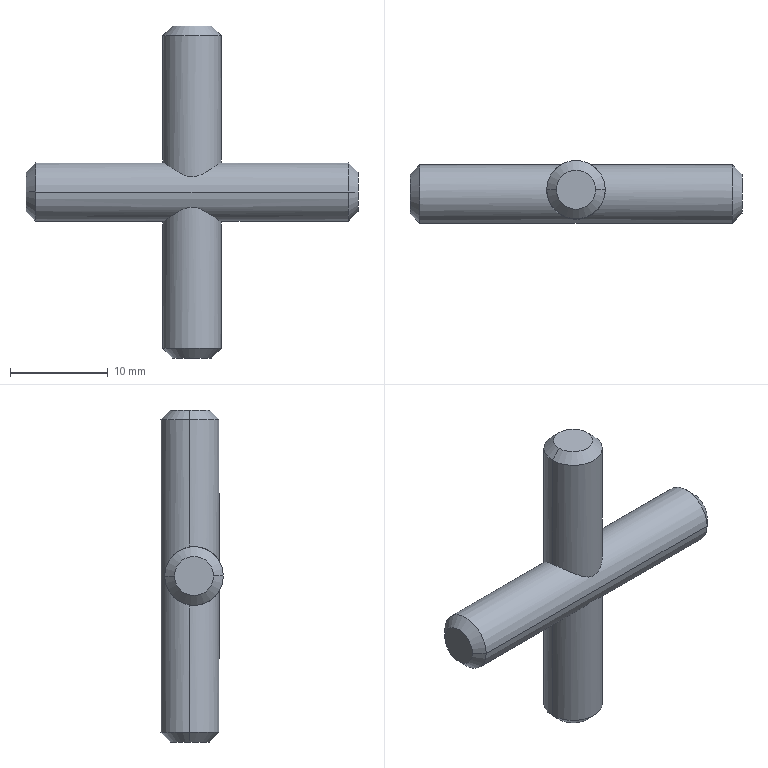Part | SolidWorks | features MBimport 1 | 1 solid | 17 faces | box 34 x 6.427 x 34 mm | volume 1749 mm3 | cone 8 | cylinder 5 | plane 4 | commonest cylinder face diameters 6 x5
STEP:
#1=CARTESIAN_POINT('',(14.,0.4269,-16.));
#2=VERTEX_POINT('',#1);
#3=CARTESIAN_POINT('',(15.,0.4269,-17.));
#4=VERTEX_POINT('',#3);
#5=CARTESIAN_POINT('',(14.5,0.4269,-16.5));
#6=DIRECTION('',(0.7071,-0.000000084,-0.7071));
#7=VECTOR('',#6,1000.);
#8=LINE('',#5,#7);
#9=EDGE_CURVE('',#2,#4,#8,.T.);
#10=ORIENTED_EDGE('',*,*,#9,.T.);
#11=CARTESIAN_POINT('',(19.,0.4269,-17.));
#12=VERTEX_POINT('',#11);
#13=CARTESIAN_POINT('',(17.,0.4269,-17.));
#14=DIRECTION('',(0.,0.,1.));
#15=DIRECTION('',(1.,0.,0.));
#16=AXIS2_PLACEMENT_3D('',#13,#14,#15);
#17=CIRCLE('',#16,2.);
#18=EDGE_CURVE('',#4,#12,#17,.T.);
#19=ORIENTED_EDGE('',*,*,#18,.T.);
#20=CARTESIAN_POINT('',(20.,0.4269,-16.));
#21=VERTEX_POINT('',#20);
#22=CARTESIAN_POINT('',(19.5,0.4269,-16.5));
#23=DIRECTION('',(-0.7071,0.,-0.7071));
#24=VECTOR('',#23,1000.);
#25=LINE('',#22,#24);
#26=EDGE_CURVE('',#21,#12,#25,.T.);
#27=ORIENTED_EDGE('',*,*,#26,.F.);
#28=CARTESIAN_POINT('',(17.,0.4269,-16.));
#29=DIRECTION('',(0.,0.,1.));
#30=DIRECTION('',(1.,0.,0.));
#31=AXIS2_PLACEMENT_3D('',#28,#29,#30);
#32=CIRCLE('',#31,3.);
#33=EDGE_CURVE('',#2,#21,#32,.T.);
#34=ORIENTED_EDGE('',*,*,#33,.F.);
#35=EDGE_LOOP('',(#10,#19,#27,#34));
#36=FACE_OUTER_BOUND('',#35,.T.);
#37=CARTESIAN_POINT('',(17.,0.4269,-18.));
#38=DIRECTION('',(0.,0.,1.));
#39=DIRECTION('',(-0.9607,0.2774,0.));
#40=AXIS2_PLACEMENT_3D('',#37,#38,#39);
#41=CONICAL_SURFACE('',#40,1.,0.7854);
#42=ADVANCED_FACE('',(#36),#41,.T.);
#43=ORIENTED_EDGE('',*,*,#26,.T.);
#44=CARTESIAN_POINT('',(17.,0.4269,-17.));
#45=DIRECTION('',(0.,0.,1.));
#46=DIRECTION('',(1.,0.,0.));
#47=AXIS2_PLACEMENT_3D('',#44,#45,#46);
#48=CIRCLE('',#47,2.);
#49=EDGE_CURVE('',#12,#4,#48,.T.);
#50=ORIENTED_EDGE('',*,*,#49,.T.);
#51=ORIENTED_EDGE('',*,*,#9,.F.);
#52=CARTESIAN_POINT('',(17.,0.4269,-16.));
#53=DIRECTION('',(0.,0.,1.));
#54=DIRECTION('',(1.,0.,0.));
#55=AXIS2_PLACEMENT_3D('',#52,#53,#54);
#56=CIRCLE('',#55,3.);
#57=EDGE_CURVE('',#21,#2,#56,.T.);
#58=ORIENTED_EDGE('',*,*,#57,.F.);
#59=EDGE_LOOP('',(#43,#50,#51,#58));
#60=FACE_OUTER_BOUND('',#59,.T.);
#61=CARTESIAN_POINT('',(17.,0.4269,-18.));
#62=DIRECTION('',(0.,0.,1.));
#63=DIRECTION('',(1.,0.,0.));
#64=AXIS2_PLACEMENT_3D('',#61,#62,#63);
#65=CONICAL_SURFACE('',#64,1.,0.7854);
#66=ADVANCED_FACE('',(#60),#65,.T.);
#67=CARTESIAN_POINT('',(14.,0.4269,-2.969));
#68=VERTEX_POINT('',#67);
#69=CARTESIAN_POINT('',(14.,0.4269,0.));
#70=DIRECTION('',(0.,0.,1.));
#71=VECTOR('',#70,1000.);
#72=LINE('',#69,#71);
#73=EDGE_CURVE('',#2,#68,#72,.T.);
#74=ORIENTED_EDGE('',*,*,#73,.T.);
#75=CARTESIAN_POINT('',(15.458,3.,0.));
#76=VERTEX_POINT('',#75);
#77=CARTESIAN_POINT('',(15.458,3.,0.));
#78=CARTESIAN_POINT('',(15.458,3.,-0.1084));
#79=CARTESIAN_POINT('',(15.449,2.995,-0.2169));
#80=CARTESIAN_POINT('',(15.433,2.985,-0.324));
#81=CARTESIAN_POINT('',(15.385,2.956,-0.541));
#82=CARTESIAN_POINT('',(15.313,2.908,-0.748));
#83=CARTESIAN_POINT('',(15.271,2.879,-0.8517));
#84=CARTESIAN_POINT('',(15.169,2.806,-1.078));
#85=CARTESIAN_POINT('',(15.055,2.713,-1.29));
#86=CARTESIAN_POINT('',(14.989,2.656,-1.404));
#87=CARTESIAN_POINT('',(14.832,2.508,-1.662));
#88=CARTESIAN_POINT('',(14.675,2.33,-1.901));
#89=CARTESIAN_POINT('',(14.587,2.218,-2.031));
#90=CARTESIAN_POINT('',(14.445,2.013,-2.237));
#91=CARTESIAN_POINT('',(14.319,1.779,-2.42));
#92=CARTESIAN_POINT('',(14.271,1.68,-2.49));
#93=CARTESIAN_POINT('',(14.182,1.472,-2.621));
#94=CARTESIAN_POINT('',(14.111,1.248,-2.733));
#95=CARTESIAN_POINT('',(14.08,1.131,-2.783));
#96=CARTESIAN_POINT('',(14.036,0.9238,-2.86));
#97=CARTESIAN_POINT('',(14.011,0.7074,-2.918));
#98=CARTESIAN_POINT('',(14.004,0.6147,-2.939));
#99=CARTESIAN_POINT('',(14.,0.5211,-2.956));
#100=CARTESIAN_POINT('',(14.,0.4269,-2.969));
#101=B_SPLINE_CURVE_WITH_KNOTS('',5,(#77,#78,#79,#80,#81,#82,#83,#84,#85,#86,#87,#88,#89,#90,#91,#92,#93,#94,#95,#96,#97,#98,#99,#100),.UNSPECIFIED.,.F.,.F.,(6,3,3,3,3,3,3,6),(0.,0.7667,1.581,2.593,3.956,4.875,5.794,6.467),.UNSPECIFIED.);
#102=EDGE_CURVE('',#76,#68,#101,.T.);
#103=ORIENTED_EDGE('',*,*,#102,.F.);
#104=CARTESIAN_POINT('',(14.,0.4269,2.969));
#105=VERTEX_POINT('',#104);
#106=CARTESIAN_POINT('',(15.458,3.,0.));
#107=CARTESIAN_POINT('',(15.458,3.,0.1084));
#108=CARTESIAN_POINT('',(15.449,2.995,0.2169));
#109=CARTESIAN_POINT('',(15.433,2.985,0.324));
#110=CARTESIAN_POINT('',(15.385,2.956,0.541));
#111=CARTESIAN_POINT('',(15.313,2.908,0.748));
#112=CARTESIAN_POINT('',(15.271,2.879,0.8517));
#113=CARTESIAN_POINT('',(15.169,2.806,1.078));
#114=CARTESIAN_POINT('',(15.055,2.713,1.29));
#115=CARTESIAN_POINT('',(14.989,2.656,1.404));
#116=CARTESIAN_POINT('',(14.832,2.508,1.662));
#117=CARTESIAN_POINT('',(14.675,2.33,1.901));
#118=CARTESIAN_POINT('',(14.587,2.218,2.031));
#119=CARTESIAN_POINT('',(14.445,2.013,2.237));
#120=CARTESIAN_POINT('',(14.319,1.779,2.42));
#121=CARTESIAN_POINT('',(14.271,1.68,2.49));
#122=CARTESIAN_POINT('',(14.182,1.472,2.621));
#123=CARTESIAN_POINT('',(14.111,1.248,2.733));
#124=CARTESIAN_POINT('',(14.08,1.131,2.783));
#125=CARTESIAN_POINT('',(14.036,0.9238,2.86));
#126=CARTESIAN_POINT('',(14.011,0.7074,2.918));
#127=CARTESIAN_POINT('',(14.004,0.6147,2.939));
#128=CARTESIAN_POINT('',(14.,0.5211,2.956));
#129=CARTESIAN_POINT('',(14.,0.4269,2.969));
#130=B_SPLINE_CURVE_WITH_KNOTS('',5,(#106,#107,#108,#109,#110,#111,#112,#113,#114,#115,#116,#117,#118,#119,#120,#121,#122,#123,#124,#125,#126,#127,#128,#129),.UNSPECIFIED.,.F.,.F.,(6,3,3,3,3,3,3,6),(0.,0.7667,1.581,2.593,3.956,4.875,5.794,6.467),.UNSPECIFIED.);
#131=EDGE_CURVE('',#76,#105,#130,.T.);
#132=ORIENTED_EDGE('',*,*,#131,.T.);
#133=CARTESIAN_POINT('',(14.,0.4269,16.));
#134=VERTEX_POINT('',#133);
#135=CARTESIAN_POINT('',(14.,0.4269,0.));
#136=DIRECTION('',(0.,0.,1.));
#137=VECTOR('',#136,1000.);
#138=LINE('',#135,#137);
#139=EDGE_CURVE('',#105,#134,#138,.T.);
#140=ORIENTED_EDGE('',*,*,#139,.T.);
#141=CARTESIAN_POINT('',(20.,0.4269,16.));
#142=VERTEX_POINT('',#141);
#143=CARTESIAN_POINT('',(17.,0.4269,16.));
#144=DIRECTION('',(0.,0.,1.));
#145=DIRECTION('',(1.,0.,0.));
#146=AXIS2_PLACEMENT_3D('',#143,#144,#145);
#147=CIRCLE('',#146,3.);
#148=EDGE_CURVE('',#142,#134,#147,.T.);
#149=ORIENTED_EDGE('',*,*,#148,.F.);
#150=CARTESIAN_POINT('',(20.,0.4269,2.969));
#151=VERTEX_POINT('',#150);
#152=CARTESIAN_POINT('',(20.,0.4269,0.));
#153=DIRECTION('',(0.,0.,1.));
#154=VECTOR('',#153,1000.);
#155=LINE('',#152,#154);
#156=EDGE_CURVE('',#151,#142,#155,.T.);
#157=ORIENTED_EDGE('',*,*,#156,.F.);
#158=CARTESIAN_POINT('',(18.542,3.,0.));
#159=VERTEX_POINT('',#158);
#160=CARTESIAN_POINT('',(18.542,3.,0.));
#161=CARTESIAN_POINT('',(18.542,3.,0.1084));
#162=CARTESIAN_POINT('',(18.551,2.995,0.2169));
#163=CARTESIAN_POINT('',(18.567,2.985,0.324));
#164=CARTESIAN_POINT('',(18.615,2.956,0.541));
#165=CARTESIAN_POINT('',(18.687,2.908,0.748));
#166=CARTESIAN_POINT('',(18.729,2.879,0.8517));
#167=CARTESIAN_POINT('',(18.831,2.806,1.078));
#168=CARTESIAN_POINT('',(18.945,2.713,1.29));
#169=CARTESIAN_POINT('',(19.011,2.656,1.404));
#170=CARTESIAN_POINT('',(19.168,2.508,1.662));
#171=CARTESIAN_POINT('',(19.325,2.33,1.901));
#172=CARTESIAN_POINT('',(19.413,2.218,2.031));
#173=CARTESIAN_POINT('',(19.555,2.013,2.237));
#174=CARTESIAN_POINT('',(19.681,1.779,2.42));
#175=CARTESIAN_POINT('',(19.729,1.68,2.49));
#176=CARTESIAN_POINT('',(19.818,1.472,2.621));
#177=CARTESIAN_POINT('',(19.889,1.248,2.733));
#178=CARTESIAN_POINT('',(19.92,1.131,2.783));
#179=CARTESIAN_POINT('',(19.964,0.9238,2.86));
#180=CARTESIAN_POINT('',(19.989,0.7074,2.918));
#181=CARTESIAN_POINT('',(19.996,0.6147,2.939));
#182=CARTESIAN_POINT('',(20.,0.5211,2.956));
#183=CARTESIAN_POINT('',(20.,0.4269,2.969));
#184=B_SPLINE_CURVE_WITH_KNOTS('',5,(#160,#161,#162,#163,#164,#165,#166,#167,#168,#169,#170,#171,#172,#173,#174,#175,#176,#177,#178,#179,#180,#181,#182,#183),.UNSPECIFIED.,.F.,.F.,(6,3,3,3,3,3,3,6),(0.,0.7667,1.581,2.593,3.956,4.875,5.794,6.467),.UNSPECIFIED.);
#185=EDGE_CURVE('',#159,#151,#184,.T.);
#186=ORIENTED_EDGE('',*,*,#185,.F.);
#187=CARTESIAN_POINT('',(20.,0.4269,-2.969));
#188=VERTEX_POINT('',#187);
#189=CARTESIAN_POINT('',(18.542,3.,0.));
#190=CARTESIAN_POINT('',(18.542,3.,-0.1084));
#191=CARTESIAN_POINT('',(18.551,2.995,-0.2169));
#192=CARTESIAN_POINT('',(18.567,2.985,-0.324));
#193=CARTESIAN_POINT('',(18.615,2.956,-0.541));
#194=CARTESIAN_POINT('',(18.687,2.908,-0.748));
#195=CARTESIAN_POINT('',(18.729,2.879,-0.8517));
#196=CARTESIAN_POINT('',(18.831,2.806,-1.078));
#197=CARTESIAN_POINT('',(18.945,2.713,-1.29));
#198=CARTESIAN_POINT('',(19.011,2.656,-1.404));
#199=CARTESIAN_POINT('',(19.168,2.508,-1.662));
#200=CARTESIAN_POINT('',(19.325,2.33,-1.901));
#201=CARTESIAN_POINT('',(19.413,2.218,-2.031));
#202=CARTESIAN_POINT('',(19.555,2.013,-2.237));
#203=CARTESIAN_POINT('',(19.681,1.779,-2.42));
#204=CARTESIAN_POINT('',(19.729,1.68,-2.49));
#205=CARTESIAN_POINT('',(19.818,1.472,-2.621));
#206=CARTESIAN_POINT('',(19.889,1.248,-2.733));
#207=CARTESIAN_POINT('',(19.92,1.131,-2.783));
#208=CARTESIAN_POINT('',(19.964,0.9238,-2.86));
#209=CARTESIAN_POINT('',(19.989,0.7074,-2.918));
#210=CARTESIAN_POINT('',(19.996,0.6147,-2.939));
#211=CARTESIAN_POINT('',(20.,0.5211,-2.956));
#212=CARTESIAN_POINT('',(20.,0.4269,-2.969));
#213=B_SPLINE_CURVE_WITH_KNOTS('',5,(#189,#190,#191,#192,#193,#194,#195,#196,#197,#198,#199,#200,#201,#202,#203,#204,#205,#206,#207,#208,#209,#210,#211,#212),.UNSPECIFIED.,.F.,.F.,(6,3,3,3,3,3,3,6),(0.,0.7667,1.581,2.593,3.956,4.875,5.794,6.467),.UNSPECIFIED.);
#214=EDGE_CURVE('',#159,#188,#213,.T.);
#215=ORIENTED_EDGE('',*,*,#214,.T.);
#216=CARTESIAN_POINT('',(20.,0.4269,0.));
#217=DIRECTION('',(0.,0.,1.));
#218=VECTOR('',#217,1000.);
#219=LINE('',#216,#218);
#220=EDGE_CURVE('',#21,#188,#219,.T.);
#221=ORIENTED_EDGE('',*,*,#220,.F.);
#222=ORIENTED_EDGE('',*,*,#57,.T.);
#223=EDGE_LOOP('',(#74,#103,#132,#140,#149,#157,#186,#215,#221,#222));
#224=FACE_OUTER_BOUND('',#223,.T.);
#225=CARTESIAN_POINT('',(17.,0.4269,0.));
#226=DIRECTION('',(0.,0.,-1.));
#227=DIRECTION('',(1.,0.,0.));
#228=AXIS2_PLACEMENT_3D('',#225,#226,#227);
#229=CYLINDRICAL_SURFACE('',#228,3.);
#230=ADVANCED_FACE('',(#224),#229,.T.);
#231=ORIENTED_EDGE('',*,*,#220,.T.);
#232=CARTESIAN_POINT('',(20.,0.4269,-2.969));
#233=CARTESIAN_POINT('',(20.,0.278,-2.991));
#234=CARTESIAN_POINT('',(19.991,0.1277,-3.003));
#235=CARTESIAN_POINT('',(19.972,-0.02222,-3.005));
#236=CARTESIAN_POINT('',(19.916,-0.3182,-2.992));
#237=CARTESIAN_POINT('',(19.824,-0.6016,-2.944));
#238=CARTESIAN_POINT('',(19.77,-0.739,-2.913));
#239=CARTESIAN_POINT('',(19.652,-0.9928,-2.838));
#240=CARTESIAN_POINT('',(19.509,-1.226,-2.742));
#241=CARTESIAN_POINT('',(19.435,-1.332,-2.692));
#242=CARTESIAN_POINT('',(19.279,-1.534,-2.584));
#243=CARTESIAN_POINT('',(19.107,-1.714,-2.465));
#244=CARTESIAN_POINT('',(19.017,-1.799,-2.404));
#245=CARTESIAN_POINT('',(18.817,-1.97,-2.269));
#246=CARTESIAN_POINT('',(18.6,-2.116,-2.13));
#247=CARTESIAN_POINT('',(18.48,-2.188,-2.056));
#248=CARTESIAN_POINT('',(18.261,-2.303,-1.927));
#249=CARTESIAN_POINT('',(18.026,-2.395,-1.808));
#250=CARTESIAN_POINT('',(17.921,-2.432,-1.759));
#251=CARTESIAN_POINT('',(17.714,-2.492,-1.672));
#252=CARTESIAN_POINT('',(17.496,-2.535,-1.605));
#253=CARTESIAN_POINT('',(17.389,-2.551,-1.579));
#254=CARTESIAN_POINT('',(17.198,-2.571,-1.547));
#255=CARTESIAN_POINT('',(17.004,-2.575,-1.54));
#256=CARTESIAN_POINT('',(16.921,-2.574,-1.541));
#257=CARTESIAN_POINT('',(16.728,-2.565,-1.557));
#258=CARTESIAN_POINT('',(16.54,-2.541,-1.596));
#259=CARTESIAN_POINT('',(16.435,-2.522,-1.625));
#260=CARTESIAN_POINT('',(16.214,-2.474,-1.699));
#261=CARTESIAN_POINT('',(16.005,-2.407,-1.793));
#262=CARTESIAN_POINT('',(15.896,-2.366,-1.846));
#263=CARTESIAN_POINT('',(15.633,-2.253,-1.986));
#264=CARTESIAN_POINT('',(15.389,-2.112,-2.136));
#265=CARTESIAN_POINT('',(15.248,-2.017,-2.227));
#266=CARTESIAN_POINT('',(15.016,-1.836,-2.381));
#267=CARTESIAN_POINT('',(14.804,-1.623,-2.527));
#268=CARTESIAN_POINT('',(14.718,-1.527,-2.586));
#269=CARTESIAN_POINT('',(14.495,-1.249,-2.74));
#270=CARTESIAN_POINT('',(14.309,-0.9305,-2.865));
#271=CARTESIAN_POINT('',(14.208,-0.7118,-2.928));
#272=CARTESIAN_POINT('',(14.087,-0.3527,-2.995));
#273=CARTESIAN_POINT('',(14.023,0.02398,-3.004));
#274=CARTESIAN_POINT('',(14.007,0.1586,-3.));
#275=CARTESIAN_POINT('',(14.,0.2933,-2.989));
#276=CARTESIAN_POINT('',(14.,0.4269,-2.969));
#277=B_SPLINE_CURVE_WITH_KNOTS('',5,(#232,#233,#234,#235,#236,#237,#238,#239,#240,#241,#242,#243,#244,#245,#246,#247,#248,#249,#250,#251,#252,#253,#254,#255,#256,#257,#258,#259,#260,#261,#262,#263,#264,#265,#266,#267,#268,#269,#270,#271,#272,#273,#274,#275,#276),.UNSPECIFIED.,.F.,.F.,(6,3,3,3,3,3,3,3,3,3,3,3,3,3,6),(0.,1.064,2.128,3.107,4.081,5.197,6.053,6.836,7.423,8.203,9.104,10.456,11.457,13.197,14.152),.UNSPECIFIED.);
#278=EDGE_CURVE('',#188,#68,#277,.T.);
#279=ORIENTED_EDGE('',*,*,#278,.T.);
#280=ORIENTED_EDGE('',*,*,#73,.F.);
#281=ORIENTED_EDGE('',*,*,#33,.T.);
#282=EDGE_LOOP('',(#231,#279,#280,#281));
#283=FACE_OUTER_BOUND('',#282,.T.);
#284=CARTESIAN_POINT('',(17.,0.4269,0.));
#285=DIRECTION('',(0.,0.,-1.));
#286=DIRECTION('',(1.,0.,0.));
#287=AXIS2_PLACEMENT_3D('',#284,#285,#286);
#288=CYLINDRICAL_SURFACE('',#287,3.);
#289=ADVANCED_FACE('',(#283),#288,.T.);
#290=ORIENTED_EDGE('',*,*,#18,.F.);
#291=ORIENTED_EDGE('',*,*,#49,.F.);
#292=EDGE_LOOP('',(#290,#291));
#293=FACE_OUTER_BOUND('',#292,.T.);
#294=CARTESIAN_POINT('',(0.,0.,-17.));
#295=DIRECTION('',(0.,0.,1.));
#296=DIRECTION('',(1.,0.,0.));
#297=AXIS2_PLACEMENT_3D('',#294,#295,#296);
#298=PLANE('',#297);
#299=ADVANCED_FACE('',(#293),#298,.F.);
#300=CARTESIAN_POINT('',(34.,-2.,-0.000000315));
#301=VERTEX_POINT('',#300);
#302=CARTESIAN_POINT('',(33.,-3.,0.));
#303=VERTEX_POINT('',#302);
#304=CARTESIAN_POINT('',(33.5,-2.5,0.));
#305=DIRECTION('',(-0.7071,-0.7071,0.));
#306=VECTOR('',#305,1000.);
#307=LINE('',#304,#306);
#308=EDGE_CURVE('',#301,#303,#307,.T.);
#309=ORIENTED_EDGE('',*,*,#308,.T.);
#310=CARTESIAN_POINT('',(33.,3.,0.));
#311=VERTEX_POINT('',#310);
#312=CARTESIAN_POINT('',(33.,0.,0.));
#313=DIRECTION('',(1.,0.,0.));
#314=DIRECTION('',(0.,1.,0.));
#315=AXIS2_PLACEMENT_3D('',#312,#313,#314);
#316=CIRCLE('',#315,3.);
#317=EDGE_CURVE('',#303,#311,#316,.T.);
#318=ORIENTED_EDGE('',*,*,#317,.T.);
#319=CARTESIAN_POINT('',(34.,2.,0.));
#320=VERTEX_POINT('',#319);
#321=CARTESIAN_POINT('',(33.5,2.5,0.));
#322=DIRECTION('',(-0.7071,0.7071,0.));
#323=VECTOR('',#322,1000.);
#324=LINE('',#321,#323);
#325=EDGE_CURVE('',#320,#311,#324,.T.);
#326=ORIENTED_EDGE('',*,*,#325,.F.);
#327=CARTESIAN_POINT('',(34.,0.,0.));
#328=DIRECTION('',(1.,0.,0.));
#329=DIRECTION('',(0.,1.,0.));
#330=AXIS2_PLACEMENT_3D('',#327,#328,#329);
#331=CIRCLE('',#330,2.);
#332=EDGE_CURVE('',#301,#320,#331,.T.);
#333=ORIENTED_EDGE('',*,*,#332,.F.);
#334=EDGE_LOOP('',(#309,#318,#326,#333));
#335=FACE_OUTER_BOUND('',#334,.T.);
#336=CARTESIAN_POINT('',(35.,0.,0.));
#337=DIRECTION('',(-1.,0.,0.));
#338=DIRECTION('',(0.,-0.809,0.5878));
#339=AXIS2_PLACEMENT_3D('',#336,#337,#338);
#340=CONICAL_SURFACE('',#339,1.,0.7854);
#341=ADVANCED_FACE('',(#335),#340,.T.);
#342=ORIENTED_EDGE('',*,*,#325,.T.);
#343=CARTESIAN_POINT('',(33.,0.,0.));
#344=DIRECTION('',(1.,0.,0.));
#345=DIRECTION('',(0.,1.,0.));
#346=AXIS2_PLACEMENT_3D('',#343,#344,#345);
#347=CIRCLE('',#346,3.);
#348=EDGE_CURVE('',#311,#303,#347,.T.);
#349=ORIENTED_EDGE('',*,*,#348,.T.);
#350=ORIENTED_EDGE('',*,*,#308,.F.);
#351=CARTESIAN_POINT('',(34.,0.,0.));
#352=DIRECTION('',(1.,0.,0.));
#353=DIRECTION('',(0.,1.,0.));
#354=AXIS2_PLACEMENT_3D('',#351,#352,#353);
#355=CIRCLE('',#354,2.);
#356=EDGE_CURVE('',#320,#301,#355,.T.);
#357=ORIENTED_EDGE('',*,*,#356,.F.);
#358=EDGE_LOOP('',(#342,#349,#350,#357));
#359=FACE_OUTER_BOUND('',#358,.T.);
#360=CARTESIAN_POINT('',(35.,0.,0.));
#361=DIRECTION('',(-1.,0.,0.));
#362=DIRECTION('',(0.,1.,0.));
#363=AXIS2_PLACEMENT_3D('',#360,#361,#362);
#364=CONICAL_SURFACE('',#363,1.,0.7854);
#365=ADVANCED_FACE('',(#359),#364,.T.);
#366=CARTESIAN_POINT('',(1.,-3.,0.));
#367=VERTEX_POINT('',#366);
#368=CARTESIAN_POINT('',(17.,-3.,0.));
#369=DIRECTION('',(1.,0.,0.));
#370=VECTOR('',#369,1000.);
#371=LINE('',#368,#370);
#372=EDGE_CURVE('',#367,#303,#371,.T.);
#373=ORIENTED_EDGE('',*,*,#372,.F.);
#374=CARTESIAN_POINT('',(1.,3.,0.));
#375=VERTEX_POINT('',#374);
#376=CARTESIAN_POINT('',(1.,0.,0.));
#377=DIRECTION('',(1.,0.,0.));
#378=DIRECTION('',(0.,1.,0.));
#379=AXIS2_PLACEMENT_3D('',#376,#377,#378);
#380=CIRCLE('',#379,3.);
#381=EDGE_CURVE('',#367,#375,#380,.T.);
#382=ORIENTED_EDGE('',*,*,#381,.T.);
#383=CARTESIAN_POINT('',(17.,3.,0.));
#384=DIRECTION('',(1.,0.,0.));
#385=VECTOR('',#384,1000.);
#386=LINE('',#383,#385);
#387=EDGE_CURVE('',#375,#76,#386,.T.);
#388=ORIENTED_EDGE('',*,*,#387,.T.);
#389=ORIENTED_EDGE('',*,*,#102,.T.);
#390=ORIENTED_EDGE('',*,*,#278,.F.);
#391=ORIENTED_EDGE('',*,*,#214,.F.);
#392=CARTESIAN_POINT('',(17.,3.,0.));
#393=DIRECTION('',(1.,0.,0.));
#394=VECTOR('',#393,1000.);
#395=LINE('',#392,#394);
#396=EDGE_CURVE('',#159,#311,#395,.T.);
#397=ORIENTED_EDGE('',*,*,#396,.T.);
#398=ORIENTED_EDGE('',*,*,#317,.F.);
#399=EDGE_LOOP('',(#373,#382,#388,#389,#390,#391,#397,#398));
#400=FACE_OUTER_BOUND('',#399,.T.);
#401=CARTESIAN_POINT('',(17.,0.,0.));
#402=DIRECTION('',(-1.,0.,0.));
#403=DIRECTION('',(0.,1.,0.));
#404=AXIS2_PLACEMENT_3D('',#401,#402,#403);
#405=CYLINDRICAL_SURFACE('',#404,3.);
#406=ADVANCED_FACE('',(#400),#405,.T.);
#407=ORIENTED_EDGE('',*,*,#396,.F.);
#408=ORIENTED_EDGE('',*,*,#185,.T.);
#409=CARTESIAN_POINT('',(14.,0.4269,2.969));
#410=CARTESIAN_POINT('',(14.,0.278,2.991));
#411=CARTESIAN_POINT('',(14.009,0.1277,3.003));
#412=CARTESIAN_POINT('',(14.028,-0.02222,3.005));
#413=CARTESIAN_POINT('',(14.084,-0.3182,2.992));
#414=CARTESIAN_POINT('',(14.176,-0.6016,2.944));
#415=CARTESIAN_POINT('',(14.23,-0.739,2.913));
#416=CARTESIAN_POINT('',(14.348,-0.9928,2.838));
#417=CARTESIAN_POINT('',(14.491,-1.226,2.742));
#418=CARTESIAN_POINT('',(14.565,-1.332,2.692));
#419=CARTESIAN_POINT('',(14.721,-1.534,2.584));
#420=CARTESIAN_POINT('',(14.893,-1.714,2.465));
#421=CARTESIAN_POINT('',(14.983,-1.799,2.404));
#422=CARTESIAN_POINT('',(15.183,-1.97,2.269));
#423=CARTESIAN_POINT('',(15.4,-2.116,2.13));
#424=CARTESIAN_POINT('',(15.52,-2.188,2.056));
#425=CARTESIAN_POINT('',(15.739,-2.303,1.927));
#426=CARTESIAN_POINT('',(15.974,-2.395,1.808));
#427=CARTESIAN_POINT('',(16.079,-2.432,1.759));
#428=CARTESIAN_POINT('',(16.286,-2.492,1.672));
#429=CARTESIAN_POINT('',(16.504,-2.535,1.605));
#430=CARTESIAN_POINT('',(16.611,-2.551,1.579));
#431=CARTESIAN_POINT('',(16.802,-2.571,1.547));
#432=CARTESIAN_POINT('',(16.996,-2.575,1.54));
#433=CARTESIAN_POINT('',(17.079,-2.574,1.541));
#434=CARTESIAN_POINT('',(17.272,-2.565,1.557));
#435=CARTESIAN_POINT('',(17.46,-2.541,1.596));
#436=CARTESIAN_POINT('',(17.565,-2.522,1.625));
#437=CARTESIAN_POINT('',(17.786,-2.474,1.699));
#438=CARTESIAN_POINT('',(17.995,-2.407,1.793));
#439=CARTESIAN_POINT('',(18.104,-2.366,1.846));
#440=CARTESIAN_POINT('',(18.367,-2.253,1.986));
#441=CARTESIAN_POINT('',(18.611,-2.112,2.136));
#442=CARTESIAN_POINT('',(18.752,-2.017,2.227));
#443=CARTESIAN_POINT('',(18.984,-1.836,2.381));
#444=CARTESIAN_POINT('',(19.196,-1.623,2.527));
#445=CARTESIAN_POINT('',(19.282,-1.527,2.586));
#446=CARTESIAN_POINT('',(19.505,-1.249,2.74));
#447=CARTESIAN_POINT('',(19.691,-0.9305,2.865));
#448=CARTESIAN_POINT('',(19.792,-0.7118,2.928));
#449=CARTESIAN_POINT('',(19.913,-0.3527,2.995));
#450=CARTESIAN_POINT('',(19.977,0.02398,3.004));
#451=CARTESIAN_POINT('',(19.993,0.1586,3.));
#452=CARTESIAN_POINT('',(20.,0.2933,2.989));
#453=CARTESIAN_POINT('',(20.,0.4269,2.969));
#454=B_SPLINE_CURVE_WITH_KNOTS('',5,(#409,#410,#411,#412,#413,#414,#415,#416,#417,#418,#419,#420,#421,#422,#423,#424,#425,#426,#427,#428,#429,#430,#431,#432,#433,#434,#435,#436,#437,#438,#439,#440,#441,#442,#443,#444,#445,#446,#447,#448,#449,#450,#451,#452,#453),.UNSPECIFIED.,.F.,.F.,(6,3,3,3,3,3,3,3,3,3,3,3,3,3,6),(0.,1.064,2.128,3.107,4.081,5.197,6.053,6.836,7.423,8.203,9.104,10.456,11.457,13.197,14.152),.UNSPECIFIED.);
#455=EDGE_CURVE('',#105,#151,#454,.T.);
#456=ORIENTED_EDGE('',*,*,#455,.F.);
#457=ORIENTED_EDGE('',*,*,#131,.F.);
#458=ORIENTED_EDGE('',*,*,#387,.F.);
#459=CARTESIAN_POINT('',(1.,0.,0.));
#460=DIRECTION('',(1.,0.,0.));
#461=DIRECTION('',(0.,1.,0.));
#462=AXIS2_PLACEMENT_3D('',#459,#460,#461);
#463=CIRCLE('',#462,3.);
#464=EDGE_CURVE('',#375,#367,#463,.T.);
#465=ORIENTED_EDGE('',*,*,#464,.T.);
#466=ORIENTED_EDGE('',*,*,#372,.T.);
#467=ORIENTED_EDGE('',*,*,#348,.F.);
#468=EDGE_LOOP('',(#407,#408,#456,#457,#458,#465,#466,#467));
#469=FACE_OUTER_BOUND('',#468,.T.);
#470=CARTESIAN_POINT('',(17.,0.,0.));
#471=DIRECTION('',(-1.,0.,0.));
#472=DIRECTION('',(0.,1.,0.));
#473=AXIS2_PLACEMENT_3D('',#470,#471,#472);
#474=CYLINDRICAL_SURFACE('',#473,3.);
#475=ADVANCED_FACE('',(#469),#474,.T.);
#476=ORIENTED_EDGE('',*,*,#356,.T.);
#477=ORIENTED_EDGE('',*,*,#332,.T.);
#478=EDGE_LOOP('',(#476,#477));
#479=FACE_OUTER_BOUND('',#478,.T.);
#480=CARTESIAN_POINT('',(34.,0.,0.));
#481=DIRECTION('',(1.,0.,0.));
#482=DIRECTION('',(0.,1.,0.));
#483=AXIS2_PLACEMENT_3D('',#480,#481,#482);
#484=PLANE('',#483);
#485=ADVANCED_FACE('',(#479),#484,.T.);
#486=CARTESIAN_POINT('',(0.,-2.,0.000000238));
#487=VERTEX_POINT('',#486);
#488=CARTESIAN_POINT('',(0.5,-2.5,0.000000298));
#489=DIRECTION('',(-0.7071,0.7071,-0.000000084));
#490=VECTOR('',#489,1000.);
#491=LINE('',#488,#490);
#492=EDGE_CURVE('',#367,#487,#491,.T.);
#493=ORIENTED_EDGE('',*,*,#492,.T.);
#494=CARTESIAN_POINT('',(0.,2.,0.));
#495=VERTEX_POINT('',#494);
#496=CARTESIAN_POINT('',(0.,0.,0.));
#497=DIRECTION('',(1.,0.,0.));
#498=DIRECTION('',(0.,1.,0.));
#499=AXIS2_PLACEMENT_3D('',#496,#497,#498);
#500=CIRCLE('',#499,2.);
#501=EDGE_CURVE('',#487,#495,#500,.T.);
#502=ORIENTED_EDGE('',*,*,#501,.T.);
#503=CARTESIAN_POINT('',(0.5,2.5,0.));
#504=DIRECTION('',(-0.7071,-0.7071,0.));
#505=VECTOR('',#504,1000.);
#506=LINE('',#503,#505);
#507=EDGE_CURVE('',#375,#495,#506,.T.);
#508=ORIENTED_EDGE('',*,*,#507,.F.);
#509=ORIENTED_EDGE('',*,*,#381,.F.);
#510=EDGE_LOOP('',(#493,#502,#508,#509));
#511=FACE_OUTER_BOUND('',#510,.T.);
#512=CARTESIAN_POINT('',(-1.,0.,0.));
#513=DIRECTION('',(1.,0.,0.));
#514=DIRECTION('',(0.,-0.9607,0.2774));
#515=AXIS2_PLACEMENT_3D('',#512,#513,#514);
#516=CONICAL_SURFACE('',#515,1.,0.7854);
#517=ADVANCED_FACE('',(#511),#516,.T.);
#518=ORIENTED_EDGE('',*,*,#507,.T.);
#519=CARTESIAN_POINT('',(0.,0.,0.));
#520=DIRECTION('',(1.,0.,0.));
#521=DIRECTION('',(0.,1.,0.));
#522=AXIS2_PLACEMENT_3D('',#519,#520,#521);
#523=CIRCLE('',#522,2.);
#524=EDGE_CURVE('',#495,#487,#523,.T.);
#525=ORIENTED_EDGE('',*,*,#524,.T.);
#526=ORIENTED_EDGE('',*,*,#492,.F.);
#527=ORIENTED_EDGE('',*,*,#464,.F.);
#528=EDGE_LOOP('',(#518,#525,#526,#527));
#529=FACE_OUTER_BOUND('',#528,.T.);
#530=CARTESIAN_POINT('',(-1.,0.,0.));
#531=DIRECTION('',(1.,0.,0.));
#532=DIRECTION('',(0.,1.,0.));
#533=AXIS2_PLACEMENT_3D('',#530,#531,#532);
#534=CONICAL_SURFACE('',#533,1.,0.7854);
#535=ADVANCED_FACE('',(#529),#534,.T.);
#536=ORIENTED_EDGE('',*,*,#501,.F.);
#537=ORIENTED_EDGE('',*,*,#524,.F.);
#538=EDGE_LOOP('',(#536,#537));
#539=FACE_OUTER_BOUND('',#538,.T.);
#540=CARTESIAN_POINT('',(0.,0.,0.));
#541=DIRECTION('',(1.,0.,0.));
#542=DIRECTION('',(0.,1.,0.));
#543=AXIS2_PLACEMENT_3D('',#540,#541,#542);
#544=PLANE('',#543);
#545=ADVANCED_FACE('',(#539),#544,.F.);
#546=CARTESIAN_POINT('',(15.,0.4269,17.));
#547=VERTEX_POINT('',#546);
#548=CARTESIAN_POINT('',(14.5,0.4269,16.5));
#549=DIRECTION('',(-0.7071,0.,-0.7071));
#550=VECTOR('',#549,1000.);
#551=LINE('',#548,#550);
#552=EDGE_CURVE('',#547,#134,#551,.T.);
#553=ORIENTED_EDGE('',*,*,#552,.T.);
#554=CARTESIAN_POINT('',(17.,0.4269,16.));
#555=DIRECTION('',(0.,0.,1.));
#556=DIRECTION('',(1.,0.,0.));
#557=AXIS2_PLACEMENT_3D('',#554,#555,#556);
#558=CIRCLE('',#557,3.);
#559=EDGE_CURVE('',#134,#142,#558,.T.);
#560=ORIENTED_EDGE('',*,*,#559,.T.);
#561=CARTESIAN_POINT('',(19.,0.4269,17.));
#562=VERTEX_POINT('',#561);
#563=CARTESIAN_POINT('',(19.5,0.4269,16.5));
#564=DIRECTION('',(0.7071,0.,-0.7071));
#565=VECTOR('',#564,1000.);
#566=LINE('',#563,#565);
#567=EDGE_CURVE('',#562,#142,#566,.T.);
#568=ORIENTED_EDGE('',*,*,#567,.F.);
#569=CARTESIAN_POINT('',(17.,0.4269,17.));
#570=DIRECTION('',(0.,0.,1.));
#571=DIRECTION('',(1.,0.,0.));
#572=AXIS2_PLACEMENT_3D('',#569,#570,#571);
#573=CIRCLE('',#572,2.);
#574=EDGE_CURVE('',#547,#562,#573,.T.);
#575=ORIENTED_EDGE('',*,*,#574,.F.);
#576=EDGE_LOOP('',(#553,#560,#568,#575));
#577=FACE_OUTER_BOUND('',#576,.T.);
#578=CARTESIAN_POINT('',(17.,0.4269,18.));
#579=DIRECTION('',(0.,0.,-1.));
#580=DIRECTION('',(-0.809,0.5878,0.));
#581=AXIS2_PLACEMENT_3D('',#578,#579,#580);
#582=CONICAL_SURFACE('',#581,1.,0.7854);
#583=ADVANCED_FACE('',(#577),#582,.T.);
#584=ORIENTED_EDGE('',*,*,#567,.T.);
#585=ORIENTED_EDGE('',*,*,#148,.T.);
#586=ORIENTED_EDGE('',*,*,#552,.F.);
#587=CARTESIAN_POINT('',(17.,0.4269,17.));
#588=DIRECTION('',(0.,0.,1.));
#589=DIRECTION('',(1.,0.,0.));
#590=AXIS2_PLACEMENT_3D('',#587,#588,#589);
#591=CIRCLE('',#590,2.);
#592=EDGE_CURVE('',#562,#547,#591,.T.);
#593=ORIENTED_EDGE('',*,*,#592,.F.);
#594=EDGE_LOOP('',(#584,#585,#586,#593));
#595=FACE_OUTER_BOUND('',#594,.T.);
#596=CARTESIAN_POINT('',(17.,0.4269,18.));
#597=DIRECTION('',(0.,0.,-1.));
#598=DIRECTION('',(1.,0.,0.));
#599=AXIS2_PLACEMENT_3D('',#596,#597,#598);
#600=CONICAL_SURFACE('',#599,1.,0.7854);
#601=ADVANCED_FACE('',(#595),#600,.T.);
#602=ORIENTED_EDGE('',*,*,#592,.T.);
#603=ORIENTED_EDGE('',*,*,#574,.T.);
#604=EDGE_LOOP('',(#602,#603));
#605=FACE_OUTER_BOUND('',#604,.T.);
#606=CARTESIAN_POINT('',(0.,0.,17.));
#607=DIRECTION('',(0.,0.,1.));
#608=DIRECTION('',(1.,0.,0.));
#609=AXIS2_PLACEMENT_3D('',#606,#607,#608);
#610=PLANE('',#609);
#611=ADVANCED_FACE('',(#605),#610,.T.);
#612=ORIENTED_EDGE('',*,*,#139,.F.);
#613=ORIENTED_EDGE('',*,*,#455,.T.);
#614=ORIENTED_EDGE('',*,*,#156,.T.);
#615=ORIENTED_EDGE('',*,*,#559,.F.);
#616=EDGE_LOOP('',(#612,#613,#614,#615));
#617=FACE_OUTER_BOUND('',#616,.T.);
#618=CARTESIAN_POINT('',(17.,0.4269,0.));
#619=DIRECTION('',(0.,0.,-1.));
#620=DIRECTION('',(1.,0.,0.));
#621=AXIS2_PLACEMENT_3D('',#618,#619,#620);
#622=CYLINDRICAL_SURFACE('',#621,3.);
#623=ADVANCED_FACE('',(#617),#622,.T.);
#624=CLOSED_SHELL('',(#42,#66,#230,#289,#299,#341,#365,#406,#475,#485,#517,#535,#545,#583,#601,#611,#623));
#625=MANIFOLD_SOLID_BREP('',#624);
#626=CARTESIAN_POINT('',(0.,0.,0.));
#627=DIRECTION('',(0.,0.,1.));
#628=DIRECTION('',(1.,0.,0.));
#629=AXIS2_PLACEMENT_3D('',#626,#627,#628);
#630=(LENGTH_UNIT()NAMED_UNIT(*)SI_UNIT(.MILLI.,.METRE.));
#631=UNCERTAINTY_MEASURE_WITH_UNIT(LENGTH_MEASURE(0.00001),#630,'','');
#632=(NAMED_UNIT(*)PLANE_ANGLE_UNIT()SI_UNIT($,.RADIAN.));
#633=(NAMED_UNIT(*)SI_UNIT($,.STERADIAN.)SOLID_ANGLE_UNIT());
#634=(GEOMETRIC_REPRESENTATION_CONTEXT(3)GLOBAL_UNCERTAINTY_ASSIGNED_CONTEXT((#631))GLOBAL_UNIT_ASSIGNED_CONTEXT((#630,#632,#633))REPRESENTATION_CONTEXT('',''));
#635=ADVANCED_BREP_SHAPE_REPRESENTATION('',(#625,#629),#634);